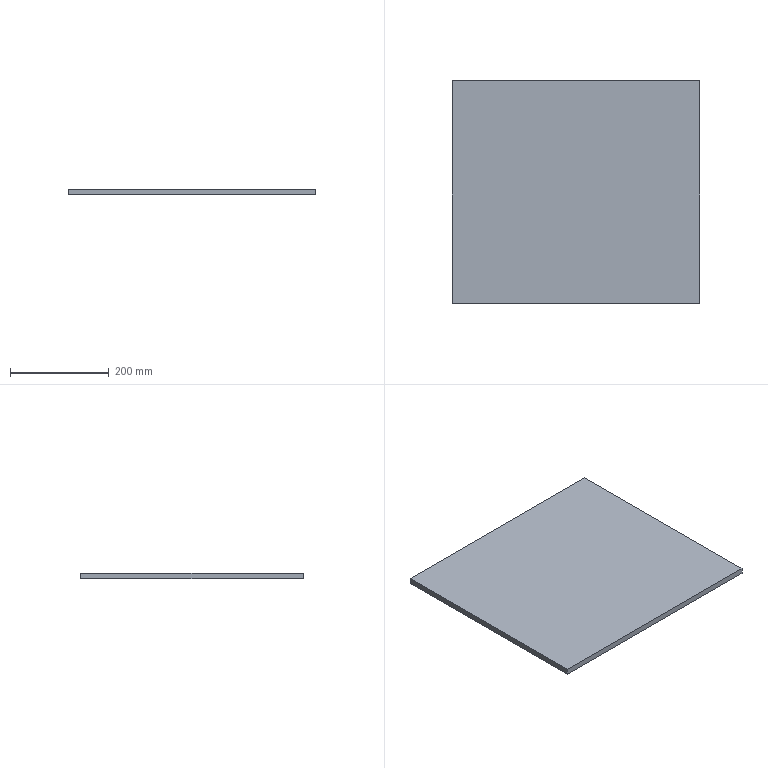Part | NX | 1 solid | 6 faces | box 500 x 450 x 12 mm | volume 2700000 mm3 | plane 6
STEP:
#1=CARTESIAN_POINT('',(-409.726,88.985,0.));
#2=VERTEX_POINT('',#1);
#3=CARTESIAN_POINT('',(90.274,88.985,0.));
#4=VERTEX_POINT('',#3);
#5=CARTESIAN_POINT('',(-369.726,88.985,0.));
#6=DIRECTION('',(1.,0.,0.));
#7=VECTOR('',#6,1000.);
#8=LINE('',#5,#7);
#9=EDGE_CURVE('',#2,#4,#8,.T.);
#10=ORIENTED_EDGE('',*,*,#9,.F.);
#11=CARTESIAN_POINT('',(-409.726,88.985,12.));
#12=VERTEX_POINT('',#11);
#13=CARTESIAN_POINT('',(-409.726,88.985,0.));
#14=DIRECTION('',(0.,0.,1.));
#15=VECTOR('',#14,1000.);
#16=LINE('',#13,#15);
#17=EDGE_CURVE('',#2,#12,#16,.T.);
#18=ORIENTED_EDGE('',*,*,#17,.T.);
#19=CARTESIAN_POINT('',(90.274,88.985,12.));
#20=VERTEX_POINT('',#19);
#21=CARTESIAN_POINT('',(-369.726,88.985,12.));
#22=DIRECTION('',(1.,0.,0.));
#23=VECTOR('',#22,1000.);
#24=LINE('',#21,#23);
#25=EDGE_CURVE('',#12,#20,#24,.T.);
#26=ORIENTED_EDGE('',*,*,#25,.T.);
#27=CARTESIAN_POINT('',(90.274,88.985,0.));
#28=DIRECTION('',(0.,0.,1.));
#29=VECTOR('',#28,1000.);
#30=LINE('',#27,#29);
#31=EDGE_CURVE('',#4,#20,#30,.T.);
#32=ORIENTED_EDGE('',*,*,#31,.F.);
#33=EDGE_LOOP('',(#10,#18,#26,#32));
#34=FACE_BOUND('',#33,.T.);
#35=CARTESIAN_POINT('',(-409.726,88.985,0.));
#36=DIRECTION('',(0.,1.,0.));
#37=DIRECTION('',(1.,0.,0.));
#38=AXIS2_PLACEMENT_3D('',#35,#36,#37);
#39=PLANE('',#38);
#40=ADVANCED_FACE('',(#34),#39,.T.);
#41=CARTESIAN_POINT('',(-409.726,-361.015,0.));
#42=VERTEX_POINT('',#41);
#43=CARTESIAN_POINT('',(-409.726,48.985,0.));
#44=DIRECTION('',(0.,-1.,0.));
#45=VECTOR('',#44,1000.);
#46=LINE('',#43,#45);
#47=EDGE_CURVE('',#2,#42,#46,.T.);
#48=ORIENTED_EDGE('',*,*,#47,.T.);
#49=CARTESIAN_POINT('',(-409.726,-361.015,12.));
#50=VERTEX_POINT('',#49);
#51=CARTESIAN_POINT('',(-409.726,-361.015,0.));
#52=DIRECTION('',(0.,0.,1.));
#53=VECTOR('',#52,1000.);
#54=LINE('',#51,#53);
#55=EDGE_CURVE('',#42,#50,#54,.T.);
#56=ORIENTED_EDGE('',*,*,#55,.T.);
#57=CARTESIAN_POINT('',(-409.726,48.985,12.));
#58=DIRECTION('',(0.,-1.,0.));
#59=VECTOR('',#58,1000.);
#60=LINE('',#57,#59);
#61=EDGE_CURVE('',#12,#50,#60,.T.);
#62=ORIENTED_EDGE('',*,*,#61,.F.);
#63=ORIENTED_EDGE('',*,*,#17,.F.);
#64=EDGE_LOOP('',(#48,#56,#62,#63));
#65=FACE_BOUND('',#64,.T.);
#66=CARTESIAN_POINT('',(-409.726,-361.015,0.));
#67=DIRECTION('',(-1.,0.,0.));
#68=DIRECTION('',(0.,0.,1.));
#69=AXIS2_PLACEMENT_3D('',#66,#67,#68);
#70=PLANE('',#69);
#71=ADVANCED_FACE('',(#65),#70,.T.);
#72=CARTESIAN_POINT('',(90.274,-361.015,0.));
#73=VERTEX_POINT('',#72);
#74=CARTESIAN_POINT('',(-369.726,-361.015,0.));
#75=DIRECTION('',(1.,0.,0.));
#76=VECTOR('',#75,1000.);
#77=LINE('',#74,#76);
#78=EDGE_CURVE('',#42,#73,#77,.T.);
#79=ORIENTED_EDGE('',*,*,#78,.T.);
#80=CARTESIAN_POINT('',(90.274,-361.015,12.));
#81=VERTEX_POINT('',#80);
#82=CARTESIAN_POINT('',(90.274,-361.015,0.));
#83=DIRECTION('',(0.,0.,1.));
#84=VECTOR('',#83,1000.);
#85=LINE('',#82,#84);
#86=EDGE_CURVE('',#73,#81,#85,.T.);
#87=ORIENTED_EDGE('',*,*,#86,.T.);
#88=CARTESIAN_POINT('',(-369.726,-361.015,12.));
#89=DIRECTION('',(1.,0.,0.));
#90=VECTOR('',#89,1000.);
#91=LINE('',#88,#90);
#92=EDGE_CURVE('',#50,#81,#91,.T.);
#93=ORIENTED_EDGE('',*,*,#92,.F.);
#94=ORIENTED_EDGE('',*,*,#55,.F.);
#95=EDGE_LOOP('',(#79,#87,#93,#94));
#96=FACE_BOUND('',#95,.T.);
#97=CARTESIAN_POINT('',(90.274,-361.015,0.));
#98=DIRECTION('',(0.,-1.,0.));
#99=DIRECTION('',(0.,0.,-1.));
#100=AXIS2_PLACEMENT_3D('',#97,#98,#99);
#101=PLANE('',#100);
#102=ADVANCED_FACE('',(#96),#101,.T.);
#103=CARTESIAN_POINT('',(90.274,48.985,0.));
#104=DIRECTION('',(0.,-1.,0.));
#105=VECTOR('',#104,1000.);
#106=LINE('',#103,#105);
#107=EDGE_CURVE('',#4,#73,#106,.T.);
#108=ORIENTED_EDGE('',*,*,#107,.F.);
#109=ORIENTED_EDGE('',*,*,#31,.T.);
#110=CARTESIAN_POINT('',(90.274,48.985,12.));
#111=DIRECTION('',(0.,-1.,0.));
#112=VECTOR('',#111,1000.);
#113=LINE('',#110,#112);
#114=EDGE_CURVE('',#20,#81,#113,.T.);
#115=ORIENTED_EDGE('',*,*,#114,.T.);
#116=ORIENTED_EDGE('',*,*,#86,.F.);
#117=EDGE_LOOP('',(#108,#109,#115,#116));
#118=FACE_BOUND('',#117,.T.);
#119=CARTESIAN_POINT('',(90.274,88.985,0.));
#120=DIRECTION('',(1.,0.,0.));
#121=DIRECTION('',(0.,1.,0.));
#122=AXIS2_PLACEMENT_3D('',#119,#120,#121);
#123=PLANE('',#122);
#124=ADVANCED_FACE('',(#118),#123,.T.);
#125=ORIENTED_EDGE('',*,*,#92,.T.);
#126=ORIENTED_EDGE('',*,*,#114,.F.);
#127=ORIENTED_EDGE('',*,*,#25,.F.);
#128=ORIENTED_EDGE('',*,*,#61,.T.);
#129=EDGE_LOOP('',(#125,#126,#127,#128));
#130=FACE_BOUND('',#129,.T.);
#131=CARTESIAN_POINT('',(-273.242,-346.647,12.));
#132=DIRECTION('',(0.,0.,1.));
#133=DIRECTION('',(1.,0.,0.));
#134=AXIS2_PLACEMENT_3D('',#131,#132,#133);
#135=PLANE('',#134);
#136=ADVANCED_FACE('',(#130),#135,.T.);
#137=ORIENTED_EDGE('',*,*,#47,.F.);
#138=ORIENTED_EDGE('',*,*,#9,.T.);
#139=ORIENTED_EDGE('',*,*,#107,.T.);
#140=ORIENTED_EDGE('',*,*,#78,.F.);
#141=EDGE_LOOP('',(#137,#138,#139,#140));
#142=FACE_BOUND('',#141,.T.);
#143=CARTESIAN_POINT('',(-273.242,-346.647,0.));
#144=DIRECTION('',(0.,0.,1.));
#145=DIRECTION('',(1.,0.,0.));
#146=AXIS2_PLACEMENT_3D('',#143,#144,#145);
#147=PLANE('',#146);
#148=ADVANCED_FACE('',(#142),#147,.F.);
#149=CLOSED_SHELL('',(#40,#71,#102,#124,#136,#148));
#150=MANIFOLD_SOLID_BREP('',#149);
#151=(LENGTH_UNIT()NAMED_UNIT(*)SI_UNIT(.MILLI.,.METRE.));
#152=UNCERTAINTY_MEASURE_WITH_UNIT(LENGTH_MEASURE(0.00001),#151,'','');
#153=(NAMED_UNIT(*)PLANE_ANGLE_UNIT()SI_UNIT($,.RADIAN.));
#154=(NAMED_UNIT(*)SI_UNIT($,.STERADIAN.)SOLID_ANGLE_UNIT());
#155=(GEOMETRIC_REPRESENTATION_CONTEXT(3)GLOBAL_UNCERTAINTY_ASSIGNED_CONTEXT((#152))GLOBAL_UNIT_ASSIGNED_CONTEXT((#151,#153,#154))REPRESENTATION_CONTEXT('',''));
#156=ADVANCED_BREP_SHAPE_REPRESENTATION('',(#150),#155);